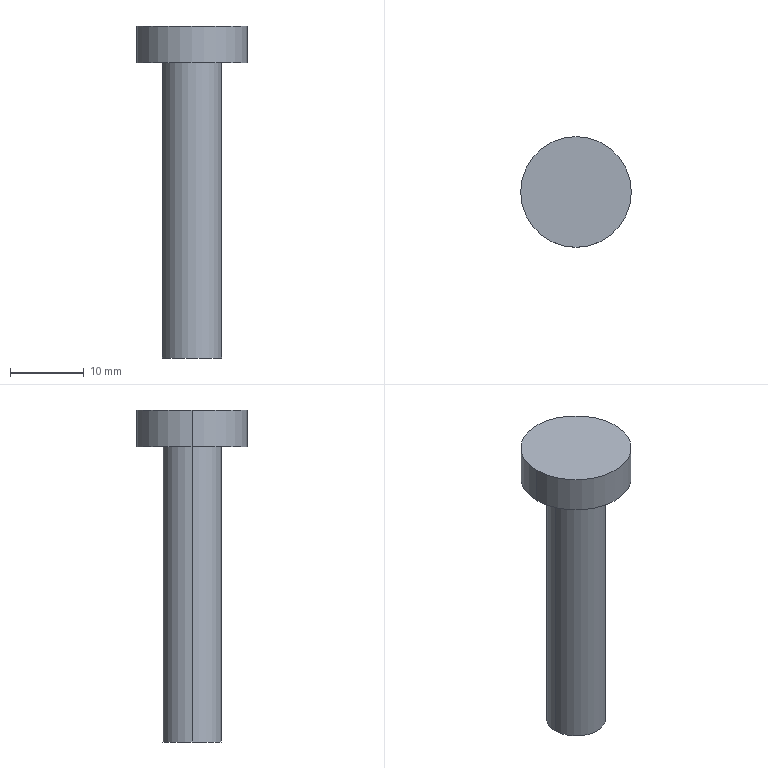Part | SolidWorks | features Extrusion 1, ICE 1 | 1 solid | 7 faces | box 15 x 15 x 45 mm | volume 2894 mm3 | cylinder 4 | plane 3 | commonest cylinder face diameters 8 x2 15 x2
STEP:
#1=CARTESIAN_POINT('',(7.5,0.,45.));
#2=VERTEX_POINT('',#1);
#3=CARTESIAN_POINT('',(-7.5,0.,45.));
#4=VERTEX_POINT('',#3);
#5=CARTESIAN_POINT('',(0.,0.,45.));
#6=DIRECTION('',(0.,0.,1.));
#7=DIRECTION('',(1.,0.,0.));
#8=AXIS2_PLACEMENT_3D('',#5,#6,#7);
#9=CIRCLE('',#8,7.5);
#10=EDGE_CURVE('',#2,#4,#9,.T.);
#11=ORIENTED_EDGE('',*,*,#10,.F.);
#12=CARTESIAN_POINT('',(7.5,0.,40.));
#13=VERTEX_POINT('',#12);
#14=CARTESIAN_POINT('',(7.5,0.,45.));
#15=DIRECTION('',(0.,0.,-1.));
#16=VECTOR('',#15,1000.);
#17=LINE('',#14,#16);
#18=EDGE_CURVE('',#2,#13,#17,.T.);
#19=ORIENTED_EDGE('',*,*,#18,.T.);
#20=CARTESIAN_POINT('',(-7.5,0.,40.));
#21=VERTEX_POINT('',#20);
#22=CARTESIAN_POINT('',(0.,0.,40.));
#23=DIRECTION('',(0.,0.,1.));
#24=DIRECTION('',(1.,0.,0.));
#25=AXIS2_PLACEMENT_3D('',#22,#23,#24);
#26=CIRCLE('',#25,7.5);
#27=EDGE_CURVE('',#13,#21,#26,.T.);
#28=ORIENTED_EDGE('',*,*,#27,.T.);
#29=CARTESIAN_POINT('',(-7.5,0.,45.));
#30=DIRECTION('',(0.,0.,-1.));
#31=VECTOR('',#30,1000.);
#32=LINE('',#29,#31);
#33=EDGE_CURVE('',#4,#21,#32,.T.);
#34=ORIENTED_EDGE('',*,*,#33,.F.);
#35=EDGE_LOOP('',(#11,#19,#28,#34));
#36=FACE_OUTER_BOUND('',#35,.T.);
#37=CARTESIAN_POINT('',(0.,0.,45.));
#38=DIRECTION('',(0.,0.,-1.));
#39=DIRECTION('',(-1.,0.,0.));
#40=AXIS2_PLACEMENT_3D('',#37,#38,#39);
#41=CYLINDRICAL_SURFACE('',#40,7.5);
#42=ADVANCED_FACE('',(#36),#41,.T.);
#43=CARTESIAN_POINT('',(4.,0.,40.));
#44=VERTEX_POINT('',#43);
#45=CARTESIAN_POINT('',(-4.,0.,40.));
#46=VERTEX_POINT('',#45);
#47=CARTESIAN_POINT('',(0.,0.,40.));
#48=DIRECTION('',(0.,0.,1.));
#49=DIRECTION('',(1.,0.,0.));
#50=AXIS2_PLACEMENT_3D('',#47,#48,#49);
#51=CIRCLE('',#50,4.);
#52=EDGE_CURVE('',#44,#46,#51,.T.);
#53=ORIENTED_EDGE('',*,*,#52,.F.);
#54=CARTESIAN_POINT('',(4.,0.,0.));
#55=VERTEX_POINT('',#54);
#56=CARTESIAN_POINT('',(4.,0.,40.));
#57=DIRECTION('',(0.,0.,-1.));
#58=VECTOR('',#57,1000.);
#59=LINE('',#56,#58);
#60=EDGE_CURVE('',#44,#55,#59,.T.);
#61=ORIENTED_EDGE('',*,*,#60,.T.);
#62=CARTESIAN_POINT('',(-4.,0.,0.));
#63=VERTEX_POINT('',#62);
#64=CARTESIAN_POINT('',(0.,0.,0.));
#65=DIRECTION('',(0.,0.,1.));
#66=DIRECTION('',(1.,0.,0.));
#67=AXIS2_PLACEMENT_3D('',#64,#65,#66);
#68=CIRCLE('',#67,4.);
#69=EDGE_CURVE('',#55,#63,#68,.T.);
#70=ORIENTED_EDGE('',*,*,#69,.T.);
#71=CARTESIAN_POINT('',(-4.,0.,40.));
#72=DIRECTION('',(0.,0.,-1.));
#73=VECTOR('',#72,1000.);
#74=LINE('',#71,#73);
#75=EDGE_CURVE('',#46,#63,#74,.T.);
#76=ORIENTED_EDGE('',*,*,#75,.F.);
#77=EDGE_LOOP('',(#53,#61,#70,#76));
#78=FACE_OUTER_BOUND('',#77,.T.);
#79=CARTESIAN_POINT('',(0.,0.,40.));
#80=DIRECTION('',(0.,0.,-1.));
#81=DIRECTION('',(-1.,0.,0.));
#82=AXIS2_PLACEMENT_3D('',#79,#80,#81);
#83=CYLINDRICAL_SURFACE('',#82,4.);
#84=ADVANCED_FACE('',(#78),#83,.T.);
#85=ORIENTED_EDGE('',*,*,#60,.F.);
#86=CARTESIAN_POINT('',(0.,0.,40.));
#87=DIRECTION('',(0.,0.,1.));
#88=DIRECTION('',(1.,0.,0.));
#89=AXIS2_PLACEMENT_3D('',#86,#87,#88);
#90=CIRCLE('',#89,4.);
#91=EDGE_CURVE('',#46,#44,#90,.T.);
#92=ORIENTED_EDGE('',*,*,#91,.F.);
#93=ORIENTED_EDGE('',*,*,#75,.T.);
#94=CARTESIAN_POINT('',(0.,0.,0.));
#95=DIRECTION('',(0.,0.,1.));
#96=DIRECTION('',(1.,0.,0.));
#97=AXIS2_PLACEMENT_3D('',#94,#95,#96);
#98=CIRCLE('',#97,4.);
#99=EDGE_CURVE('',#63,#55,#98,.T.);
#100=ORIENTED_EDGE('',*,*,#99,.T.);
#101=EDGE_LOOP('',(#85,#92,#93,#100));
#102=FACE_OUTER_BOUND('',#101,.T.);
#103=CARTESIAN_POINT('',(0.,0.,40.));
#104=DIRECTION('',(0.,0.,-1.));
#105=DIRECTION('',(-1.,0.,0.));
#106=AXIS2_PLACEMENT_3D('',#103,#104,#105);
#107=CYLINDRICAL_SURFACE('',#106,4.);
#108=ADVANCED_FACE('',(#102),#107,.T.);
#109=ORIENTED_EDGE('',*,*,#99,.F.);
#110=ORIENTED_EDGE('',*,*,#69,.F.);
#111=EDGE_LOOP('',(#109,#110));
#112=FACE_OUTER_BOUND('',#111,.T.);
#113=CARTESIAN_POINT('',(0.,0.,0.));
#114=DIRECTION('',(0.,0.,1.));
#115=DIRECTION('',(1.,0.,0.));
#116=AXIS2_PLACEMENT_3D('',#113,#114,#115);
#117=PLANE('',#116);
#118=ADVANCED_FACE('',(#112),#117,.F.);
#119=ORIENTED_EDGE('',*,*,#18,.F.);
#120=CARTESIAN_POINT('',(0.,0.,45.));
#121=DIRECTION('',(0.,0.,1.));
#122=DIRECTION('',(1.,0.,0.));
#123=AXIS2_PLACEMENT_3D('',#120,#121,#122);
#124=CIRCLE('',#123,7.5);
#125=EDGE_CURVE('',#4,#2,#124,.T.);
#126=ORIENTED_EDGE('',*,*,#125,.F.);
#127=ORIENTED_EDGE('',*,*,#33,.T.);
#128=CARTESIAN_POINT('',(0.,0.,40.));
#129=DIRECTION('',(0.,0.,1.));
#130=DIRECTION('',(1.,0.,0.));
#131=AXIS2_PLACEMENT_3D('',#128,#129,#130);
#132=CIRCLE('',#131,7.5);
#133=EDGE_CURVE('',#21,#13,#132,.T.);
#134=ORIENTED_EDGE('',*,*,#133,.T.);
#135=EDGE_LOOP('',(#119,#126,#127,#134));
#136=FACE_OUTER_BOUND('',#135,.T.);
#137=CARTESIAN_POINT('',(0.,0.,45.));
#138=DIRECTION('',(0.,0.,-1.));
#139=DIRECTION('',(-1.,0.,0.));
#140=AXIS2_PLACEMENT_3D('',#137,#138,#139);
#141=CYLINDRICAL_SURFACE('',#140,7.5);
#142=ADVANCED_FACE('',(#136),#141,.T.);
#143=ORIENTED_EDGE('',*,*,#125,.T.);
#144=ORIENTED_EDGE('',*,*,#10,.T.);
#145=EDGE_LOOP('',(#143,#144));
#146=FACE_OUTER_BOUND('',#145,.T.);
#147=CARTESIAN_POINT('',(0.,0.,45.));
#148=DIRECTION('',(0.,0.,1.));
#149=DIRECTION('',(1.,0.,0.));
#150=AXIS2_PLACEMENT_3D('',#147,#148,#149);
#151=PLANE('',#150);
#152=ADVANCED_FACE('',(#146),#151,.T.);
#153=ORIENTED_EDGE('',*,*,#91,.T.);
#154=ORIENTED_EDGE('',*,*,#52,.T.);
#155=EDGE_LOOP('',(#153,#154));
#156=FACE_BOUND('',#155,.T.);
#157=ORIENTED_EDGE('',*,*,#133,.F.);
#158=ORIENTED_EDGE('',*,*,#27,.F.);
#159=EDGE_LOOP('',(#157,#158));
#160=FACE_OUTER_BOUND('',#159,.T.);
#161=CARTESIAN_POINT('',(0.,0.,40.));
#162=DIRECTION('',(0.,0.,1.));
#163=DIRECTION('',(1.,0.,0.));
#164=AXIS2_PLACEMENT_3D('',#161,#162,#163);
#165=PLANE('',#164);
#166=ADVANCED_FACE('',(#156,#160),#165,.F.);
#167=CLOSED_SHELL('',(#42,#84,#108,#118,#142,#152,#166));
#168=MANIFOLD_SOLID_BREP('',#167);
#169=CARTESIAN_POINT('',(0.,0.,0.));
#170=DIRECTION('',(0.,0.,1.));
#171=DIRECTION('',(1.,0.,0.));
#172=AXIS2_PLACEMENT_3D('',#169,#170,#171);
#173=(LENGTH_UNIT()NAMED_UNIT(*)SI_UNIT(.MILLI.,.METRE.));
#174=UNCERTAINTY_MEASURE_WITH_UNIT(LENGTH_MEASURE(0.00001),#173,'','');
#175=(NAMED_UNIT(*)PLANE_ANGLE_UNIT()SI_UNIT($,.RADIAN.));
#176=(NAMED_UNIT(*)SI_UNIT($,.STERADIAN.)SOLID_ANGLE_UNIT());
#177=(GEOMETRIC_REPRESENTATION_CONTEXT(3)GLOBAL_UNCERTAINTY_ASSIGNED_CONTEXT((#174))GLOBAL_UNIT_ASSIGNED_CONTEXT((#173,#175,#176))REPRESENTATION_CONTEXT('',''));
#178=ADVANCED_BREP_SHAPE_REPRESENTATION('',(#168,#172),#177);